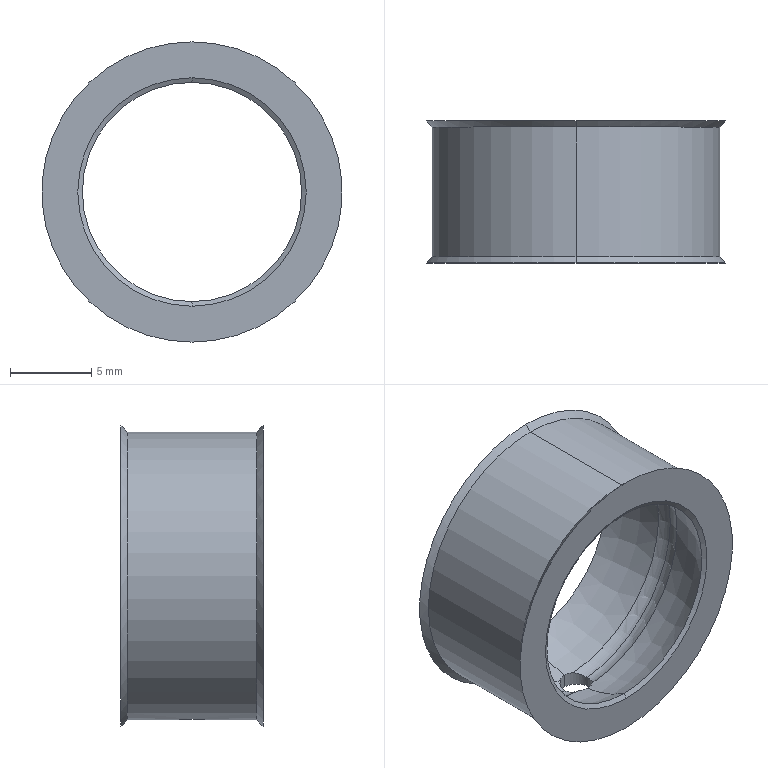Part | NX | features LUMP3 2 | 1 solid | 22 faces | box 18.466 x 8.738 x 18.466 mm | volume 562.765 mm3 | cone 8 | torus 8 | cylinder 4 | plane 2 | commonest cylinder face diameters 1.981 x2 17.704 x2
STEP:
#1=CARTESIAN_POINT('',(0.,4.369,25.692));
#2=VERTEX_POINT('',#1);
#3=CARTESIAN_POINT('',(0.,3.988,26.073));
#4=VERTEX_POINT('',#3);
#5=CARTESIAN_POINT('',(0.,4.178,25.883));
#6=DIRECTION('',(0.,-0.7071,0.7071));
#7=VECTOR('',#6,1000.);
#8=LINE('',#5,#7);
#9=EDGE_CURVE('',#2,#4,#8,.T.);
#10=ORIENTED_EDGE('',*,*,#9,.T.);
#11=CARTESIAN_POINT('',(0.,3.988,43.777));
#12=VERTEX_POINT('',#11);
#13=CARTESIAN_POINT('',(0.,3.988,34.925));
#14=DIRECTION('',(0.,-1.,0.));
#15=DIRECTION('',(0.,0.,-1.));
#16=AXIS2_PLACEMENT_3D('',#13,#14,#15);
#17=CIRCLE('',#16,8.852);
#18=EDGE_CURVE('',#12,#4,#17,.T.);
#19=ORIENTED_EDGE('',*,*,#18,.F.);
#20=CARTESIAN_POINT('',(0.,4.369,44.158));
#21=VERTEX_POINT('',#20);
#22=CARTESIAN_POINT('',(0.,4.178,43.967));
#23=DIRECTION('',(0.,0.7071,0.7071));
#24=VECTOR('',#23,1000.);
#25=LINE('',#22,#24);
#26=EDGE_CURVE('',#12,#21,#25,.T.);
#27=ORIENTED_EDGE('',*,*,#26,.T.);
#28=CARTESIAN_POINT('',(0.,4.369,34.925));
#29=DIRECTION('',(0.,-1.,0.));
#30=DIRECTION('',(0.,0.,-1.));
#31=AXIS2_PLACEMENT_3D('',#28,#29,#30);
#32=CIRCLE('',#31,9.233);
#33=EDGE_CURVE('',#21,#2,#32,.T.);
#34=ORIENTED_EDGE('',*,*,#33,.T.);
#35=EDGE_LOOP('',(#10,#19,#27,#34));
#36=FACE_BOUND('',#35,.T.);
#37=CARTESIAN_POINT('',(0.,4.178,34.925));
#38=DIRECTION('',(0.,1.,0.));
#39=DIRECTION('',(0.,0.,1.));
#40=AXIS2_PLACEMENT_3D('',#37,#38,#39);
#41=CONICAL_SURFACE('',#40,9.042,0.7854);
#42=ADVANCED_FACE('',(#36),#41,.T.);
#43=CARTESIAN_POINT('',(0.,-4.369,44.158));
#44=VERTEX_POINT('',#43);
#45=CARTESIAN_POINT('',(0.,-3.988,43.777));
#46=VERTEX_POINT('',#45);
#47=CARTESIAN_POINT('',(0.,-4.178,43.967));
#48=DIRECTION('',(0.,0.7071,-0.7071));
#49=VECTOR('',#48,1000.);
#50=LINE('',#47,#49);
#51=EDGE_CURVE('',#44,#46,#50,.T.);
#52=ORIENTED_EDGE('',*,*,#51,.T.);
#53=CARTESIAN_POINT('',(0.,-3.988,26.073));
#54=VERTEX_POINT('',#53);
#55=CARTESIAN_POINT('',(0.,-3.988,34.925));
#56=DIRECTION('',(0.,1.,0.));
#57=DIRECTION('',(0.,0.,-1.));
#58=AXIS2_PLACEMENT_3D('',#55,#56,#57);
#59=CIRCLE('',#58,8.852);
#60=EDGE_CURVE('',#54,#46,#59,.T.);
#61=ORIENTED_EDGE('',*,*,#60,.F.);
#62=CARTESIAN_POINT('',(0.,-4.369,25.692));
#63=VERTEX_POINT('',#62);
#64=CARTESIAN_POINT('',(0.,-4.178,25.883));
#65=DIRECTION('',(0.,-0.7071,-0.7071));
#66=VECTOR('',#65,1000.);
#67=LINE('',#64,#66);
#68=EDGE_CURVE('',#54,#63,#67,.T.);
#69=ORIENTED_EDGE('',*,*,#68,.T.);
#70=CARTESIAN_POINT('',(0.,-4.369,34.925));
#71=DIRECTION('',(0.,1.,0.));
#72=DIRECTION('',(0.,0.,1.));
#73=AXIS2_PLACEMENT_3D('',#70,#71,#72);
#74=CIRCLE('',#73,9.233);
#75=EDGE_CURVE('',#63,#44,#74,.T.);
#76=ORIENTED_EDGE('',*,*,#75,.T.);
#77=EDGE_LOOP('',(#52,#61,#69,#76));
#78=FACE_BOUND('',#77,.T.);
#79=CARTESIAN_POINT('',(0.,-4.178,34.925));
#80=DIRECTION('',(0.,-1.,0.));
#81=DIRECTION('',(0.,0.,-1.));
#82=AXIS2_PLACEMENT_3D('',#79,#80,#81);
#83=CONICAL_SURFACE('',#82,9.042,0.7854);
#84=ADVANCED_FACE('',(#78),#83,.T.);
#85=CARTESIAN_POINT('',(0.,4.369,34.925));
#86=DIRECTION('',(0.,-1.,0.));
#87=DIRECTION('',(0.,0.,-1.));
#88=AXIS2_PLACEMENT_3D('',#85,#86,#87);
#89=CIRCLE('',#88,9.233);
#90=EDGE_CURVE('',#2,#21,#89,.T.);
#91=ORIENTED_EDGE('',*,*,#90,.F.);
#92=ORIENTED_EDGE('',*,*,#33,.F.);
#93=EDGE_LOOP('',(#91,#92));
#94=FACE_BOUND('',#93,.T.);
#95=CARTESIAN_POINT('',(0.,4.369,27.901));
#96=VERTEX_POINT('',#95);
#97=CARTESIAN_POINT('',(0.,4.369,41.949));
#98=VERTEX_POINT('',#97);
#99=CARTESIAN_POINT('',(0.,4.369,34.925));
#100=DIRECTION('',(0.,-1.,0.));
#101=DIRECTION('',(0.,0.,-1.));
#102=AXIS2_PLACEMENT_3D('',#99,#100,#101);
#103=CIRCLE('',#102,7.024);
#104=EDGE_CURVE('',#96,#98,#103,.T.);
#105=ORIENTED_EDGE('',*,*,#104,.T.);
#106=CARTESIAN_POINT('',(0.,4.369,34.925));
#107=DIRECTION('',(0.,-1.,0.));
#108=DIRECTION('',(0.,0.,-1.));
#109=AXIS2_PLACEMENT_3D('',#106,#107,#108);
#110=CIRCLE('',#109,7.024);
#111=EDGE_CURVE('',#98,#96,#110,.T.);
#112=ORIENTED_EDGE('',*,*,#111,.T.);
#113=EDGE_LOOP('',(#105,#112));
#114=FACE_BOUND('',#113,.T.);
#115=CARTESIAN_POINT('',(0.,4.369,34.925));
#116=DIRECTION('',(0.,1.,0.));
#117=DIRECTION('',(-1.,0.,0.));
#118=AXIS2_PLACEMENT_3D('',#115,#116,#117);
#119=PLANE('',#118);
#120=ADVANCED_FACE('',(#94,#114),#119,.T.);
#121=CARTESIAN_POINT('',(0.,4.205,28.184));
#122=VERTEX_POINT('',#121);
#123=CARTESIAN_POINT('',(0.,4.254,28.1));
#124=DIRECTION('',(0.,-0.5,0.866));
#125=VECTOR('',#124,1000.);
#126=LINE('',#123,#125);
#127=EDGE_CURVE('',#96,#122,#126,.T.);
#128=ORIENTED_EDGE('',*,*,#127,.F.);
#129=ORIENTED_EDGE('',*,*,#111,.F.);
#130=CARTESIAN_POINT('',(0.,4.205,41.666));
#131=VERTEX_POINT('',#130);
#132=CARTESIAN_POINT('',(0.,4.254,41.75));
#133=DIRECTION('',(0.,0.5,0.866));
#134=VECTOR('',#133,1000.);
#135=LINE('',#132,#134);
#136=EDGE_CURVE('',#131,#98,#135,.T.);
#137=ORIENTED_EDGE('',*,*,#136,.F.);
#138=CARTESIAN_POINT('',(0.,4.205,34.925));
#139=DIRECTION('',(0.,1.,0.));
#140=DIRECTION('',(0.,0.,-1.));
#141=AXIS2_PLACEMENT_3D('',#138,#139,#140);
#142=CIRCLE('',#141,6.741);
#143=EDGE_CURVE('',#122,#131,#142,.T.);
#144=ORIENTED_EDGE('',*,*,#143,.F.);
#145=EDGE_LOOP('',(#128,#129,#137,#144));
#146=FACE_BOUND('',#145,.T.);
#147=CARTESIAN_POINT('',(0.,4.254,34.925));
#148=DIRECTION('',(0.,1.,0.));
#149=DIRECTION('',(0.,0.,1.));
#150=AXIS2_PLACEMENT_3D('',#147,#148,#149);
#151=CONICAL_SURFACE('',#150,6.825,1.047);
#152=ADVANCED_FACE('',(#146),#151,.F.);
#153=CARTESIAN_POINT('',(0.,-4.369,34.925));
#154=DIRECTION('',(0.,1.,0.));
#155=DIRECTION('',(0.,0.,1.));
#156=AXIS2_PLACEMENT_3D('',#153,#154,#155);
#157=CIRCLE('',#156,9.233);
#158=EDGE_CURVE('',#44,#63,#157,.T.);
#159=ORIENTED_EDGE('',*,*,#158,.F.);
#160=ORIENTED_EDGE('',*,*,#75,.F.);
#161=EDGE_LOOP('',(#159,#160));
#162=FACE_BOUND('',#161,.T.);
#163=CARTESIAN_POINT('',(0.,-4.369,27.901));
#164=VERTEX_POINT('',#163);
#165=CARTESIAN_POINT('',(0.,-4.369,41.949));
#166=VERTEX_POINT('',#165);
#167=CARTESIAN_POINT('',(0.,-4.369,34.925));
#168=DIRECTION('',(0.,1.,0.));
#169=DIRECTION('',(0.,0.,-1.));
#170=AXIS2_PLACEMENT_3D('',#167,#168,#169);
#171=CIRCLE('',#170,7.024);
#172=EDGE_CURVE('',#164,#166,#171,.T.);
#173=ORIENTED_EDGE('',*,*,#172,.T.);
#174=CARTESIAN_POINT('',(0.,-4.369,34.925));
#175=DIRECTION('',(0.,1.,0.));
#176=DIRECTION('',(0.,0.,-1.));
#177=AXIS2_PLACEMENT_3D('',#174,#175,#176);
#178=CIRCLE('',#177,7.024);
#179=EDGE_CURVE('',#166,#164,#178,.T.);
#180=ORIENTED_EDGE('',*,*,#179,.T.);
#181=EDGE_LOOP('',(#173,#180));
#182=FACE_BOUND('',#181,.T.);
#183=CARTESIAN_POINT('',(0.,-4.369,34.925));
#184=DIRECTION('',(0.,-1.,0.));
#185=DIRECTION('',(-1.,0.,0.));
#186=AXIS2_PLACEMENT_3D('',#183,#184,#185);
#187=PLANE('',#186);
#188=ADVANCED_FACE('',(#162,#182),#187,.T.);
#189=CARTESIAN_POINT('',(0.,-4.205,28.184));
#190=VERTEX_POINT('',#189);
#191=CARTESIAN_POINT('',(0.,-4.254,28.1));
#192=DIRECTION('',(0.,0.5,0.866));
#193=VECTOR('',#192,1000.);
#194=LINE('',#191,#193);
#195=EDGE_CURVE('',#164,#190,#194,.T.);
#196=ORIENTED_EDGE('',*,*,#195,.T.);
#197=CARTESIAN_POINT('',(0.,-4.205,41.666));
#198=VERTEX_POINT('',#197);
#199=CARTESIAN_POINT('',(0.,-4.205,34.925));
#200=DIRECTION('',(0.,-1.,0.));
#201=DIRECTION('',(0.,0.,-1.));
#202=AXIS2_PLACEMENT_3D('',#199,#200,#201);
#203=CIRCLE('',#202,6.741);
#204=EDGE_CURVE('',#198,#190,#203,.T.);
#205=ORIENTED_EDGE('',*,*,#204,.F.);
#206=CARTESIAN_POINT('',(0.,-4.254,41.75));
#207=DIRECTION('',(0.,-0.5,0.866));
#208=VECTOR('',#207,1000.);
#209=LINE('',#206,#208);
#210=EDGE_CURVE('',#198,#166,#209,.T.);
#211=ORIENTED_EDGE('',*,*,#210,.T.);
#212=ORIENTED_EDGE('',*,*,#172,.F.);
#213=EDGE_LOOP('',(#196,#205,#211,#212));
#214=FACE_BOUND('',#213,.T.);
#215=CARTESIAN_POINT('',(0.,-4.254,34.925));
#216=DIRECTION('',(0.,-1.,0.));
#217=DIRECTION('',(0.,0.,1.));
#218=AXIS2_PLACEMENT_3D('',#215,#216,#217);
#219=CONICAL_SURFACE('',#218,6.825,1.047);
#220=ADVANCED_FACE('',(#214),#219,.F.);
#221=ORIENTED_EDGE('',*,*,#51,.F.);
#222=ORIENTED_EDGE('',*,*,#158,.T.);
#223=ORIENTED_EDGE('',*,*,#68,.F.);
#224=CARTESIAN_POINT('',(0.,-3.988,34.925));
#225=DIRECTION('',(0.,1.,0.));
#226=DIRECTION('',(0.,0.,-1.));
#227=AXIS2_PLACEMENT_3D('',#224,#225,#226);
#228=CIRCLE('',#227,8.852);
#229=EDGE_CURVE('',#46,#54,#228,.T.);
#230=ORIENTED_EDGE('',*,*,#229,.F.);
#231=EDGE_LOOP('',(#221,#222,#223,#230));
#232=FACE_BOUND('',#231,.T.);
#233=CARTESIAN_POINT('',(0.,-4.178,34.925));
#234=DIRECTION('',(0.,-1.,0.));
#235=DIRECTION('',(0.,0.,-1.));
#236=AXIS2_PLACEMENT_3D('',#233,#234,#235);
#237=CONICAL_SURFACE('',#236,9.042,0.7854);
#238=ADVANCED_FACE('',(#232),#237,.T.);
#239=ORIENTED_EDGE('',*,*,#9,.F.);
#240=ORIENTED_EDGE('',*,*,#90,.T.);
#241=ORIENTED_EDGE('',*,*,#26,.F.);
#242=CARTESIAN_POINT('',(0.,3.988,34.925));
#243=DIRECTION('',(0.,-1.,0.));
#244=DIRECTION('',(0.,0.,-1.));
#245=AXIS2_PLACEMENT_3D('',#242,#243,#244);
#246=CIRCLE('',#245,8.852);
#247=EDGE_CURVE('',#4,#12,#246,.T.);
#248=ORIENTED_EDGE('',*,*,#247,.F.);
#249=EDGE_LOOP('',(#239,#240,#241,#248));
#250=FACE_BOUND('',#249,.T.);
#251=CARTESIAN_POINT('',(0.,4.178,34.925));
#252=DIRECTION('',(0.,1.,0.));
#253=DIRECTION('',(0.,0.,1.));
#254=AXIS2_PLACEMENT_3D('',#251,#252,#253);
#255=CONICAL_SURFACE('',#254,9.042,0.7854);
#256=ADVANCED_FACE('',(#250),#255,.T.);
#257=CARTESIAN_POINT('',(0.,-0.9906,26.073));
#258=VERTEX_POINT('',#257);
#259=CARTESIAN_POINT('',(0.,0.,26.073));
#260=DIRECTION('',(0.,1.,0.));
#261=VECTOR('',#260,1000.);
#262=LINE('',#259,#261);
#263=EDGE_CURVE('',#54,#258,#262,.T.);
#264=ORIENTED_EDGE('',*,*,#263,.F.);
#265=ORIENTED_EDGE('',*,*,#60,.T.);
#266=CARTESIAN_POINT('',(0.,0.,43.777));
#267=DIRECTION('',(0.,-1.,0.));
#268=VECTOR('',#267,1000.);
#269=LINE('',#266,#268);
#270=EDGE_CURVE('',#12,#46,#269,.T.);
#271=ORIENTED_EDGE('',*,*,#270,.F.);
#272=ORIENTED_EDGE('',*,*,#18,.T.);
#273=CARTESIAN_POINT('',(0.,0.9906,26.073));
#274=VERTEX_POINT('',#273);
#275=CARTESIAN_POINT('',(0.,0.,26.073));
#276=DIRECTION('',(0.,1.,0.));
#277=VECTOR('',#276,1000.);
#278=LINE('',#275,#277);
#279=EDGE_CURVE('',#274,#4,#278,.T.);
#280=ORIENTED_EDGE('',*,*,#279,.F.);
#281=CARTESIAN_POINT('',(-0.9906,0.,26.129));
#282=VERTEX_POINT('',#281);
#283=CARTESIAN_POINT('',(0.,0.9906,26.073));
#284=CARTESIAN_POINT('',(-0.5237,0.9906,26.073));
#285=CARTESIAN_POINT('',(-0.9906,0.5237,26.129));
#286=CARTESIAN_POINT('',(-0.9906,0.,26.129));
#287=B_SPLINE_CURVE_WITH_KNOTS('',3,(#283,#284,#285,#286),.UNSPECIFIED.,.F.,.F.,(4,4),(0.,0.001549),.UNSPECIFIED.);
#288=EDGE_CURVE('',#274,#282,#287,.T.);
#289=ORIENTED_EDGE('',*,*,#288,.T.);
#290=CARTESIAN_POINT('',(-0.9906,0.,26.129));
#291=CARTESIAN_POINT('',(-0.9906,-0.5237,26.129));
#292=CARTESIAN_POINT('',(-0.5237,-0.9906,26.073));
#293=CARTESIAN_POINT('',(0.,-0.9906,26.073));
#294=B_SPLINE_CURVE_WITH_KNOTS('',3,(#290,#291,#292,#293),.UNSPECIFIED.,.F.,.F.,(4,4),(0.,0.001549),.UNSPECIFIED.);
#295=EDGE_CURVE('',#282,#258,#294,.T.);
#296=ORIENTED_EDGE('',*,*,#295,.T.);
#297=EDGE_LOOP('',(#264,#265,#271,#272,#280,#289,#296));
#298=FACE_BOUND('',#297,.T.);
#299=CARTESIAN_POINT('',(0.,0.,34.925));
#300=DIRECTION('',(0.,1.,0.));
#301=DIRECTION('',(0.,0.,1.));
#302=AXIS2_PLACEMENT_3D('',#299,#300,#301);
#303=CYLINDRICAL_SURFACE('',#302,8.852);
#304=ADVANCED_FACE('',(#298),#303,.T.);
#305=ORIENTED_EDGE('',*,*,#127,.T.);
#306=CARTESIAN_POINT('',(0.,4.205,34.925));
#307=DIRECTION('',(0.,1.,0.));
#308=DIRECTION('',(0.,0.,-1.));
#309=AXIS2_PLACEMENT_3D('',#306,#307,#308);
#310=CIRCLE('',#309,6.741);
#311=EDGE_CURVE('',#131,#122,#310,.T.);
#312=ORIENTED_EDGE('',*,*,#311,.F.);
#313=ORIENTED_EDGE('',*,*,#136,.T.);
#314=ORIENTED_EDGE('',*,*,#104,.F.);
#315=EDGE_LOOP('',(#305,#312,#313,#314));
#316=FACE_BOUND('',#315,.T.);
#317=CARTESIAN_POINT('',(0.,4.254,34.925));
#318=DIRECTION('',(0.,1.,0.));
#319=DIRECTION('',(0.,0.,1.));
#320=AXIS2_PLACEMENT_3D('',#317,#318,#319);
#321=CONICAL_SURFACE('',#320,6.825,1.047);
#322=ADVANCED_FACE('',(#316),#321,.F.);
#323=CARTESIAN_POINT('',(0.,0.8041,42.908));
#324=VERTEX_POINT('',#323);
#325=CARTESIAN_POINT('',(0.,0.,35.433));
#326=DIRECTION('',(-1.,0.,0.));
#327=DIRECTION('',(0.,0.,1.));
#328=AXIS2_PLACEMENT_3D('',#325,#326,#327);
#329=CIRCLE('',#328,7.519);
#330=EDGE_CURVE('',#324,#131,#329,.T.);
#331=ORIENTED_EDGE('',*,*,#330,.F.);
#332=CARTESIAN_POINT('',(-0.5786,0.8041,26.963));
#333=VERTEX_POINT('',#332);
#334=CARTESIAN_POINT('',(0.,0.8041,34.925));
#335=DIRECTION('',(0.,-1.,0.));
#336=DIRECTION('',(0.,0.,1.));
#337=AXIS2_PLACEMENT_3D('',#334,#335,#336);
#338=CIRCLE('',#337,7.983);
#339=EDGE_CURVE('',#324,#333,#338,.T.);
#340=ORIENTED_EDGE('',*,*,#339,.T.);
#341=CARTESIAN_POINT('',(0.,0.9906,26.964));
#342=VERTEX_POINT('',#341);
#343=CARTESIAN_POINT('',(-0.5786,0.8041,26.963));
#344=CARTESIAN_POINT('',(-0.5714,0.8092,26.963));
#345=CARTESIAN_POINT('',(-0.5642,0.8143,26.963));
#346=CARTESIAN_POINT('',(-0.4682,0.8796,26.963));
#347=CARTESIAN_POINT('',(-0.3702,0.9251,26.963));
#348=CARTESIAN_POINT('',(-0.18,0.9783,26.964));
#349=CARTESIAN_POINT('',(-0.09019,0.9906,26.964));
#350=CARTESIAN_POINT('',(0.,0.9906,26.964));
#351=B_SPLINE_CURVE_WITH_KNOTS('',3,(#343,#344,#345,#346,#347,#348,#349,#350),.UNSPECIFIED.,.F.,.F.,(4,2,2,4),(0.,0.04274,0.5629,1.),.UNSPECIFIED.);
#352=EDGE_CURVE('',#333,#342,#351,.T.);
#353=ORIENTED_EDGE('',*,*,#352,.T.);
#354=CARTESIAN_POINT('',(0.,0.,34.417));
#355=DIRECTION('',(-1.,0.,0.));
#356=DIRECTION('',(0.,0.,-1.));
#357=AXIS2_PLACEMENT_3D('',#354,#355,#356);
#358=CIRCLE('',#357,7.519);
#359=EDGE_CURVE('',#122,#342,#358,.T.);
#360=ORIENTED_EDGE('',*,*,#359,.F.);
#361=ORIENTED_EDGE('',*,*,#143,.T.);
#362=EDGE_LOOP('',(#331,#340,#353,#360,#361));
#363=FACE_BOUND('',#362,.T.);
#364=CARTESIAN_POINT('',(0.,0.,34.925));
#365=DIRECTION('',(0.,-1.,0.));
#366=DIRECTION('',(1.,0.,0.));
#367=AXIS2_PLACEMENT_3D('',#364,#365,#366);
#368=DEGENERATE_TOROIDAL_SURFACE('',#367,0.508,7.519,.T.);
#369=ADVANCED_FACE('',(#363),#368,.F.);
#370=ORIENTED_EDGE('',*,*,#195,.F.);
#371=ORIENTED_EDGE('',*,*,#179,.F.);
#372=ORIENTED_EDGE('',*,*,#210,.F.);
#373=CARTESIAN_POINT('',(0.,-4.205,34.925));
#374=DIRECTION('',(0.,-1.,0.));
#375=DIRECTION('',(0.,0.,-1.));
#376=AXIS2_PLACEMENT_3D('',#373,#374,#375);
#377=CIRCLE('',#376,6.741);
#378=EDGE_CURVE('',#190,#198,#377,.T.);
#379=ORIENTED_EDGE('',*,*,#378,.F.);
#380=EDGE_LOOP('',(#370,#371,#372,#379));
#381=FACE_BOUND('',#380,.T.);
#382=CARTESIAN_POINT('',(0.,-4.254,34.925));
#383=DIRECTION('',(0.,-1.,0.));
#384=DIRECTION('',(0.,0.,1.));
#385=AXIS2_PLACEMENT_3D('',#382,#383,#384);
#386=CONICAL_SURFACE('',#385,6.825,1.047);
#387=ADVANCED_FACE('',(#381),#386,.F.);
#388=CARTESIAN_POINT('',(0.,-0.8041,42.908));
#389=VERTEX_POINT('',#388);
#390=CARTESIAN_POINT('',(0.,0.,35.433));
#391=DIRECTION('',(-1.,0.,0.));
#392=DIRECTION('',(0.,0.,1.));
#393=AXIS2_PLACEMENT_3D('',#390,#391,#392);
#394=CIRCLE('',#393,7.519);
#395=EDGE_CURVE('',#198,#389,#394,.T.);
#396=ORIENTED_EDGE('',*,*,#395,.F.);
#397=ORIENTED_EDGE('',*,*,#204,.T.);
#398=CARTESIAN_POINT('',(0.,-0.9906,26.964));
#399=VERTEX_POINT('',#398);
#400=CARTESIAN_POINT('',(0.,0.,34.417));
#401=DIRECTION('',(-1.,0.,0.));
#402=DIRECTION('',(0.,0.,-1.));
#403=AXIS2_PLACEMENT_3D('',#400,#401,#402);
#404=CIRCLE('',#403,7.519);
#405=EDGE_CURVE('',#399,#190,#404,.T.);
#406=ORIENTED_EDGE('',*,*,#405,.F.);
#407=CARTESIAN_POINT('',(-0.5786,-0.8041,26.963));
#408=VERTEX_POINT('',#407);
#409=CARTESIAN_POINT('',(0.,-0.9906,26.964));
#410=CARTESIAN_POINT('',(-0.08915,-0.9906,26.964));
#411=CARTESIAN_POINT('',(-0.1779,-0.9786,26.964));
#412=CARTESIAN_POINT('',(-0.367,-0.9263,26.963));
#413=CARTESIAN_POINT('',(-0.4649,-0.8813,26.963));
#414=CARTESIAN_POINT('',(-0.562,-0.8158,26.963));
#415=CARTESIAN_POINT('',(-0.5703,-0.81,26.963));
#416=CARTESIAN_POINT('',(-0.5786,-0.8041,26.963));
#417=B_SPLINE_CURVE_WITH_KNOTS('',3,(#409,#410,#411,#412,#413,#414,#415,#416),.UNSPECIFIED.,.F.,.F.,(4,2,2,4),(0.,0.4321,0.9508,1.),.UNSPECIFIED.);
#418=EDGE_CURVE('',#399,#408,#417,.T.);
#419=ORIENTED_EDGE('',*,*,#418,.T.);
#420=CARTESIAN_POINT('',(0.,-0.8041,34.925));
#421=DIRECTION('',(0.,1.,0.));
#422=DIRECTION('',(0.,0.,1.));
#423=AXIS2_PLACEMENT_3D('',#420,#421,#422);
#424=CIRCLE('',#423,7.983);
#425=EDGE_CURVE('',#408,#389,#424,.T.);
#426=ORIENTED_EDGE('',*,*,#425,.T.);
#427=EDGE_LOOP('',(#396,#397,#406,#419,#426));
#428=FACE_BOUND('',#427,.T.);
#429=CARTESIAN_POINT('',(0.,0.,34.925));
#430=DIRECTION('',(0.,-1.,0.));
#431=DIRECTION('',(1.,0.,0.));
#432=AXIS2_PLACEMENT_3D('',#429,#430,#431);
#433=DEGENERATE_TOROIDAL_SURFACE('',#432,0.508,7.519,.T.);
#434=ADVANCED_FACE('',(#428),#433,.F.);
#435=ORIENTED_EDGE('',*,*,#263,.T.);
#436=CARTESIAN_POINT('',(0.,-0.9906,26.073));
#437=CARTESIAN_POINT('',(0.5239,-0.9906,26.073));
#438=CARTESIAN_POINT('',(1.457,-0.001423,26.184));
#439=CARTESIAN_POINT('',(0.5239,0.9906,26.073));
#440=CARTESIAN_POINT('',(0.,0.9906,26.073));
#441=B_SPLINE_CURVE_WITH_KNOTS('',3,(#436,#437,#438,#439,#440),.UNSPECIFIED.,.F.,.F.,(4,1,4),(0.,0.001549,0.003099),.UNSPECIFIED.);
#442=EDGE_CURVE('',#258,#274,#441,.T.);
#443=ORIENTED_EDGE('',*,*,#442,.T.);
#444=ORIENTED_EDGE('',*,*,#279,.T.);
#445=ORIENTED_EDGE('',*,*,#247,.T.);
#446=ORIENTED_EDGE('',*,*,#270,.T.);
#447=ORIENTED_EDGE('',*,*,#229,.T.);
#448=EDGE_LOOP('',(#435,#443,#444,#445,#446,#447));
#449=FACE_BOUND('',#448,.T.);
#450=CARTESIAN_POINT('',(0.,0.,34.925));
#451=DIRECTION('',(0.,1.,0.));
#452=DIRECTION('',(0.,0.,1.));
#453=AXIS2_PLACEMENT_3D('',#450,#451,#452);
#454=CYLINDRICAL_SURFACE('',#453,8.852);
#455=ADVANCED_FACE('',(#449),#454,.T.);
#456=CARTESIAN_POINT('',(0.,-0.9906,25.26));
#457=DIRECTION('',(0.,0.,1.));
#458=VECTOR('',#457,1000.);
#459=LINE('',#456,#458);
#460=EDGE_CURVE('',#258,#399,#459,.T.);
#461=ORIENTED_EDGE('',*,*,#460,.F.);
#462=ORIENTED_EDGE('',*,*,#295,.F.);
#463=ORIENTED_EDGE('',*,*,#288,.F.);
#464=CARTESIAN_POINT('',(0.,0.9906,25.26));
#465=DIRECTION('',(0.,0.,-1.));
#466=VECTOR('',#465,1000.);
#467=LINE('',#464,#466);
#468=EDGE_CURVE('',#342,#274,#467,.T.);
#469=ORIENTED_EDGE('',*,*,#468,.F.);
#470=ORIENTED_EDGE('',*,*,#352,.F.);
#471=CARTESIAN_POINT('',(-0.9906,0.,26.781));
#472=VERTEX_POINT('',#471);
#473=CARTESIAN_POINT('',(-0.5786,0.8041,26.963));
#474=CARTESIAN_POINT('',(-0.8301,0.6231,26.873));
#475=CARTESIAN_POINT('',(-0.9906,0.3231,26.781));
#476=CARTESIAN_POINT('',(-0.9906,0.,26.781));
#477=B_SPLINE_CURVE_WITH_KNOTS('',3,(#473,#474,#475,#476),.UNSPECIFIED.,.F.,.F.,(4,4),(0.,0.0009544),.UNSPECIFIED.);
#478=EDGE_CURVE('',#333,#472,#477,.T.);
#479=ORIENTED_EDGE('',*,*,#478,.T.);
#480=CARTESIAN_POINT('',(-0.9906,0.,26.781));
#481=CARTESIAN_POINT('',(-0.9906,-0.323,26.781));
#482=CARTESIAN_POINT('',(-0.83,-0.6232,26.873));
#483=CARTESIAN_POINT('',(-0.5786,-0.8041,26.963));
#484=B_SPLINE_CURVE_WITH_KNOTS('',3,(#480,#481,#482,#483),.UNSPECIFIED.,.F.,.F.,(4,4),(0.,0.0009542),.UNSPECIFIED.);
#485=EDGE_CURVE('',#472,#408,#484,.T.);
#486=ORIENTED_EDGE('',*,*,#485,.T.);
#487=ORIENTED_EDGE('',*,*,#418,.F.);
#488=EDGE_LOOP('',(#461,#462,#463,#469,#470,#479,#486,#487));
#489=FACE_BOUND('',#488,.T.);
#490=CARTESIAN_POINT('',(0.,0.,25.26));
#491=DIRECTION('',(0.,0.,-1.));
#492=DIRECTION('',(0.,1.,0.));
#493=AXIS2_PLACEMENT_3D('',#490,#491,#492);
#494=CYLINDRICAL_SURFACE('',#493,0.9906);
#495=ADVANCED_FACE('',(#489),#494,.F.);
#496=ORIENTED_EDGE('',*,*,#330,.T.);
#497=ORIENTED_EDGE('',*,*,#311,.T.);
#498=ORIENTED_EDGE('',*,*,#359,.T.);
#499=CARTESIAN_POINT('',(0.5786,0.8041,26.963));
#500=VERTEX_POINT('',#499);
#501=CARTESIAN_POINT('',(0.,0.9906,26.964));
#502=CARTESIAN_POINT('',(0.088,0.9906,26.964));
#503=CARTESIAN_POINT('',(0.1756,0.9789,26.964));
#504=CARTESIAN_POINT('',(0.3635,0.9277,26.963));
#505=CARTESIAN_POINT('',(0.4612,0.8832,26.963));
#506=CARTESIAN_POINT('',(0.5596,0.8175,26.963));
#507=CARTESIAN_POINT('',(0.5692,0.8109,26.963));
#508=CARTESIAN_POINT('',(0.5786,0.8041,26.963));
#509=B_SPLINE_CURVE_WITH_KNOTS('',3,(#501,#502,#503,#504,#505,#506,#507,#508),.UNSPECIFIED.,.F.,.F.,(4,2,2,4),(0.,0.4265,0.9437,1.),.UNSPECIFIED.);
#510=EDGE_CURVE('',#342,#500,#509,.T.);
#511=ORIENTED_EDGE('',*,*,#510,.T.);
#512=CARTESIAN_POINT('',(0.,0.8041,34.925));
#513=DIRECTION('',(0.,-1.,0.));
#514=DIRECTION('',(0.,0.,1.));
#515=AXIS2_PLACEMENT_3D('',#512,#513,#514);
#516=CIRCLE('',#515,7.983);
#517=EDGE_CURVE('',#500,#324,#516,.T.);
#518=ORIENTED_EDGE('',*,*,#517,.T.);
#519=EDGE_LOOP('',(#496,#497,#498,#511,#518));
#520=FACE_BOUND('',#519,.T.);
#521=CARTESIAN_POINT('',(0.,0.,34.925));
#522=DIRECTION('',(0.,-1.,0.));
#523=DIRECTION('',(1.,0.,0.));
#524=AXIS2_PLACEMENT_3D('',#521,#522,#523);
#525=DEGENERATE_TOROIDAL_SURFACE('',#524,0.508,7.519,.T.);
#526=ADVANCED_FACE('',(#520),#525,.F.);
#527=CARTESIAN_POINT('',(0.,0.,43.129));
#528=VERTEX_POINT('',#527);
#529=CARTESIAN_POINT('',(0.,0.,34.925));
#530=DIRECTION('',(0.,-1.,0.));
#531=DIRECTION('',(0.,0.,1.));
#532=AXIS2_PLACEMENT_3D('',#529,#530,#531);
#533=CIRCLE('',#532,8.204);
#534=EDGE_CURVE('',#528,#472,#533,.T.);
#535=ORIENTED_EDGE('',*,*,#534,.T.);
#536=ORIENTED_EDGE('',*,*,#478,.F.);
#537=ORIENTED_EDGE('',*,*,#339,.F.);
#538=CARTESIAN_POINT('',(0.,0.,41.554));
#539=DIRECTION('',(-1.,0.,0.));
#540=DIRECTION('',(0.,0.,1.));
#541=AXIS2_PLACEMENT_3D('',#538,#539,#540);
#542=CIRCLE('',#541,1.575);
#543=EDGE_CURVE('',#528,#324,#542,.T.);
#544=ORIENTED_EDGE('',*,*,#543,.F.);
#545=EDGE_LOOP('',(#535,#536,#537,#544));
#546=FACE_BOUND('',#545,.T.);
#547=CARTESIAN_POINT('',(0.,0.,34.925));
#548=DIRECTION('',(0.,1.,0.));
#549=DIRECTION('',(0.,0.,1.));
#550=AXIS2_PLACEMENT_3D('',#547,#548,#549);
#551=TOROIDAL_SURFACE('',#550,6.629,1.575);
#552=ADVANCED_FACE('',(#546),#551,.F.);
#553=ORIENTED_EDGE('',*,*,#534,.F.);
#554=CARTESIAN_POINT('',(0.,0.,41.554));
#555=DIRECTION('',(-1.,0.,0.));
#556=DIRECTION('',(0.,0.,1.));
#557=AXIS2_PLACEMENT_3D('',#554,#555,#556);
#558=CIRCLE('',#557,1.575);
#559=EDGE_CURVE('',#389,#528,#558,.T.);
#560=ORIENTED_EDGE('',*,*,#559,.F.);
#561=ORIENTED_EDGE('',*,*,#425,.F.);
#562=ORIENTED_EDGE('',*,*,#485,.F.);
#563=EDGE_LOOP('',(#553,#560,#561,#562));
#564=FACE_BOUND('',#563,.T.);
#565=CARTESIAN_POINT('',(0.,0.,34.925));
#566=DIRECTION('',(0.,1.,0.));
#567=DIRECTION('',(0.,0.,1.));
#568=AXIS2_PLACEMENT_3D('',#565,#566,#567);
#569=TOROIDAL_SURFACE('',#568,6.629,1.575);
#570=ADVANCED_FACE('',(#564),#569,.F.);
#571=ORIENTED_EDGE('',*,*,#395,.T.);
#572=CARTESIAN_POINT('',(0.5786,-0.8041,26.963));
#573=VERTEX_POINT('',#572);
#574=CARTESIAN_POINT('',(0.,-0.8041,34.925));
#575=DIRECTION('',(0.,1.,0.));
#576=DIRECTION('',(0.,0.,1.));
#577=AXIS2_PLACEMENT_3D('',#574,#575,#576);
#578=CIRCLE('',#577,7.983);
#579=EDGE_CURVE('',#389,#573,#578,.T.);
#580=ORIENTED_EDGE('',*,*,#579,.T.);
#581=CARTESIAN_POINT('',(0.5786,-0.8041,26.963));
#582=CARTESIAN_POINT('',(0.5725,-0.8084,26.963));
#583=CARTESIAN_POINT('',(0.5664,-0.8127,26.963));
#584=CARTESIAN_POINT('',(0.4715,-0.8778,26.963));
#585=CARTESIAN_POINT('',(0.3734,-0.9238,26.963));
#586=CARTESIAN_POINT('',(0.183,-0.9777,26.964));
#587=CARTESIAN_POINT('',(0.09314,-0.9903,26.964));
#588=CARTESIAN_POINT('',(0.001903,-0.9906,26.964));
#589=CARTESIAN_POINT('',(0.0009513,-0.9906,26.964));
#590=CARTESIAN_POINT('',(0.,-0.9906,26.964));
#591=B_SPLINE_CURVE_WITH_KNOTS('',3,(#581,#582,#583,#584,#585,#586,#587,#588,#589,#590),.UNSPECIFIED.,.F.,.F.,(4,2,2,2,4),(0.,0.03627,0.5578,0.9954,1.),.UNSPECIFIED.);
#592=EDGE_CURVE('',#573,#399,#591,.T.);
#593=ORIENTED_EDGE('',*,*,#592,.T.);
#594=ORIENTED_EDGE('',*,*,#405,.T.);
#595=ORIENTED_EDGE('',*,*,#378,.T.);
#596=EDGE_LOOP('',(#571,#580,#593,#594,#595));
#597=FACE_BOUND('',#596,.T.);
#598=CARTESIAN_POINT('',(0.,0.,34.925));
#599=DIRECTION('',(0.,-1.,0.));
#600=DIRECTION('',(1.,0.,0.));
#601=AXIS2_PLACEMENT_3D('',#598,#599,#600);
#602=DEGENERATE_TOROIDAL_SURFACE('',#601,0.508,7.519,.T.);
#603=ADVANCED_FACE('',(#597),#602,.F.);
#604=ORIENTED_EDGE('',*,*,#460,.T.);
#605=ORIENTED_EDGE('',*,*,#592,.F.);
#606=CARTESIAN_POINT('',(0.9906,0.,26.781));
#607=VERTEX_POINT('',#606);
#608=CARTESIAN_POINT('',(0.5786,-0.8041,26.963));
#609=CARTESIAN_POINT('',(0.8301,-0.6231,26.873));
#610=CARTESIAN_POINT('',(0.9906,-0.3231,26.781));
#611=CARTESIAN_POINT('',(0.9906,0.,26.781));
#612=B_SPLINE_CURVE_WITH_KNOTS('',3,(#608,#609,#610,#611),.UNSPECIFIED.,.F.,.F.,(4,4),(0.,0.0009544),.UNSPECIFIED.);
#613=EDGE_CURVE('',#573,#607,#612,.T.);
#614=ORIENTED_EDGE('',*,*,#613,.T.);
#615=CARTESIAN_POINT('',(0.9906,0.,26.781));
#616=CARTESIAN_POINT('',(0.9906,0.323,26.781));
#617=CARTESIAN_POINT('',(0.83,0.6232,26.873));
#618=CARTESIAN_POINT('',(0.5786,0.8041,26.963));
#619=B_SPLINE_CURVE_WITH_KNOTS('',3,(#615,#616,#617,#618),.UNSPECIFIED.,.F.,.F.,(4,4),(0.,0.0009542),.UNSPECIFIED.);
#620=EDGE_CURVE('',#607,#500,#619,.T.);
#621=ORIENTED_EDGE('',*,*,#620,.T.);
#622=ORIENTED_EDGE('',*,*,#510,.F.);
#623=ORIENTED_EDGE('',*,*,#468,.T.);
#624=ORIENTED_EDGE('',*,*,#442,.F.);
#625=EDGE_LOOP('',(#604,#605,#614,#621,#622,#623,#624));
#626=FACE_BOUND('',#625,.T.);
#627=CARTESIAN_POINT('',(0.,0.,25.26));
#628=DIRECTION('',(0.,0.,-1.));
#629=DIRECTION('',(0.,1.,0.));
#630=AXIS2_PLACEMENT_3D('',#627,#628,#629);
#631=CYLINDRICAL_SURFACE('',#630,0.9906);
#632=ADVANCED_FACE('',(#626),#631,.F.);
#633=CARTESIAN_POINT('',(0.,0.,34.925));
#634=DIRECTION('',(0.,-1.,0.));
#635=DIRECTION('',(0.,0.,1.));
#636=AXIS2_PLACEMENT_3D('',#633,#634,#635);
#637=CIRCLE('',#636,8.204);
#638=EDGE_CURVE('',#607,#528,#637,.T.);
#639=ORIENTED_EDGE('',*,*,#638,.T.);
#640=ORIENTED_EDGE('',*,*,#543,.T.);
#641=ORIENTED_EDGE('',*,*,#517,.F.);
#642=ORIENTED_EDGE('',*,*,#620,.F.);
#643=EDGE_LOOP('',(#639,#640,#641,#642));
#644=FACE_BOUND('',#643,.T.);
#645=CARTESIAN_POINT('',(0.,0.,34.925));
#646=DIRECTION('',(0.,1.,0.));
#647=DIRECTION('',(0.,0.,1.));
#648=AXIS2_PLACEMENT_3D('',#645,#646,#647);
#649=TOROIDAL_SURFACE('',#648,6.629,1.575);
#650=ADVANCED_FACE('',(#644),#649,.F.);
#651=ORIENTED_EDGE('',*,*,#638,.F.);
#652=ORIENTED_EDGE('',*,*,#613,.F.);
#653=ORIENTED_EDGE('',*,*,#579,.F.);
#654=ORIENTED_EDGE('',*,*,#559,.T.);
#655=EDGE_LOOP('',(#651,#652,#653,#654));
#656=FACE_BOUND('',#655,.T.);
#657=CARTESIAN_POINT('',(0.,0.,34.925));
#658=DIRECTION('',(0.,1.,0.));
#659=DIRECTION('',(0.,0.,1.));
#660=AXIS2_PLACEMENT_3D('',#657,#658,#659);
#661=TOROIDAL_SURFACE('',#660,6.629,1.575);
#662=ADVANCED_FACE('',(#656),#661,.F.);
#663=CLOSED_SHELL('',(#42,#84,#120,#152,#188,#220,#238,#256,#304,#322,#369,#387,#434,#455,#495,#526,#552,#570,#603,#632,#650,#662));
#664=MANIFOLD_SOLID_BREP('',#663);
#665=(LENGTH_UNIT()NAMED_UNIT(*)SI_UNIT(.MILLI.,.METRE.));
#666=UNCERTAINTY_MEASURE_WITH_UNIT(LENGTH_MEASURE(0.0508),#665,'','');
#667=(NAMED_UNIT(*)PLANE_ANGLE_UNIT()SI_UNIT($,.RADIAN.));
#668=(NAMED_UNIT(*)SI_UNIT($,.STERADIAN.)SOLID_ANGLE_UNIT());
#669=(GEOMETRIC_REPRESENTATION_CONTEXT(3)GLOBAL_UNCERTAINTY_ASSIGNED_CONTEXT((#666))GLOBAL_UNIT_ASSIGNED_CONTEXT((#665,#667,#668))REPRESENTATION_CONTEXT('',''));
#670=ADVANCED_BREP_SHAPE_REPRESENTATION('',(#664),#669);